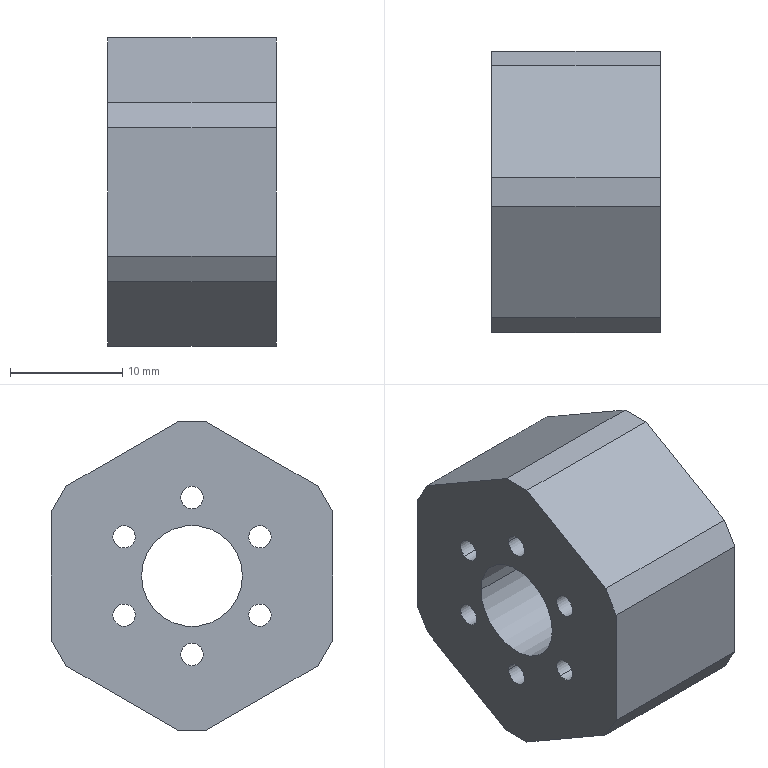Part | STEP file | ZHUANZITIEX_6_1_2_1_1 | 1 solid | 28 faces | box 15 x 25.116 x 27.5 mm | volume 6869 mm3 | plane 14 | cylinder 14 | commonest cylinder face diameters 2 x12 9 x2
STEP:
#1=CARTESIAN_POINT('',(0.,0.,0.));
#2=DIRECTION('',(0.,0.,1.));
#3=DIRECTION('',(1.,0.,0.));
#4=AXIS2_PLACEMENT_3D('',#1,#2,#3);
#5=CARTESIAN_POINT('',(0.,1.3,-13.75));
#6=VERTEX_POINT('',#5);
#7=CARTESIAN_POINT('',(0.,11.258,-8.001));
#8=VERTEX_POINT('',#7);
#9=CARTESIAN_POINT('',(0.,1.3,-13.75));
#10=DIRECTION('',(0.,0.866,0.5));
#11=VECTOR('',#10,11.498);
#12=LINE('',#9,#11);
#13=EDGE_CURVE('',#6,#8,#12,.T.);
#14=ORIENTED_EDGE('',*,*,#13,.T.);
#15=CARTESIAN_POINT('',(0.,12.558,-5.749));
#16=VERTEX_POINT('',#15);
#17=CARTESIAN_POINT('',(0.,11.258,-8.001));
#18=DIRECTION('',(0.,0.5,0.866));
#19=VECTOR('',#18,2.6);
#20=LINE('',#17,#19);
#21=EDGE_CURVE('',#8,#16,#20,.T.);
#22=ORIENTED_EDGE('',*,*,#21,.T.);
#23=CARTESIAN_POINT('',(0.,12.558,5.749));
#24=VERTEX_POINT('',#23);
#25=CARTESIAN_POINT('',(0.,12.558,-5.749));
#26=DIRECTION('',(0.,0.,1.));
#27=VECTOR('',#26,11.498);
#28=LINE('',#25,#27);
#29=EDGE_CURVE('',#16,#24,#28,.T.);
#30=ORIENTED_EDGE('',*,*,#29,.T.);
#31=CARTESIAN_POINT('',(0.,11.258,8.001));
#32=VERTEX_POINT('',#31);
#33=CARTESIAN_POINT('',(0.,12.558,5.749));
#34=DIRECTION('',(0.,-0.5,0.866));
#35=VECTOR('',#34,2.6);
#36=LINE('',#33,#35);
#37=EDGE_CURVE('',#24,#32,#36,.T.);
#38=ORIENTED_EDGE('',*,*,#37,.T.);
#39=CARTESIAN_POINT('',(0.,1.3,13.75));
#40=VERTEX_POINT('',#39);
#41=CARTESIAN_POINT('',(0.,11.258,8.001));
#42=DIRECTION('',(0.,-0.866,0.5));
#43=VECTOR('',#42,11.498);
#44=LINE('',#41,#43);
#45=EDGE_CURVE('',#32,#40,#44,.T.);
#46=ORIENTED_EDGE('',*,*,#45,.T.);
#47=CARTESIAN_POINT('',(0.,-1.3,13.75));
#48=VERTEX_POINT('',#47);
#49=CARTESIAN_POINT('',(0.,1.3,13.75));
#50=DIRECTION('',(0.,-1.,0.));
#51=VECTOR('',#50,2.6);
#52=LINE('',#49,#51);
#53=EDGE_CURVE('',#40,#48,#52,.T.);
#54=ORIENTED_EDGE('',*,*,#53,.T.);
#55=CARTESIAN_POINT('',(0.,-11.258,8.001));
#56=VERTEX_POINT('',#55);
#57=CARTESIAN_POINT('',(0.,-1.3,13.75));
#58=DIRECTION('',(0.,-0.866,-0.5));
#59=VECTOR('',#58,11.498);
#60=LINE('',#57,#59);
#61=EDGE_CURVE('',#48,#56,#60,.T.);
#62=ORIENTED_EDGE('',*,*,#61,.T.);
#63=CARTESIAN_POINT('',(0.,-12.558,5.749));
#64=VERTEX_POINT('',#63);
#65=CARTESIAN_POINT('',(0.,-11.258,8.001));
#66=DIRECTION('',(0.,-0.5,-0.866));
#67=VECTOR('',#66,2.6);
#68=LINE('',#65,#67);
#69=EDGE_CURVE('',#56,#64,#68,.T.);
#70=ORIENTED_EDGE('',*,*,#69,.T.);
#71=CARTESIAN_POINT('',(0.,-12.558,-5.749));
#72=VERTEX_POINT('',#71);
#73=CARTESIAN_POINT('',(0.,-12.558,5.749));
#74=DIRECTION('',(0.,0.,-1.));
#75=VECTOR('',#74,11.498);
#76=LINE('',#73,#75);
#77=EDGE_CURVE('',#64,#72,#76,.T.);
#78=ORIENTED_EDGE('',*,*,#77,.T.);
#79=CARTESIAN_POINT('',(0.,-11.258,-8.001));
#80=VERTEX_POINT('',#79);
#81=CARTESIAN_POINT('',(0.,-12.558,-5.749));
#82=DIRECTION('',(0.,0.5,-0.866));
#83=VECTOR('',#82,2.6);
#84=LINE('',#81,#83);
#85=EDGE_CURVE('',#72,#80,#84,.T.);
#86=ORIENTED_EDGE('',*,*,#85,.T.);
#87=CARTESIAN_POINT('',(0.,-1.3,-13.75));
#88=VERTEX_POINT('',#87);
#89=CARTESIAN_POINT('',(0.,-11.258,-8.001));
#90=DIRECTION('',(0.,0.866,-0.5));
#91=VECTOR('',#90,11.498);
#92=LINE('',#89,#91);
#93=EDGE_CURVE('',#80,#88,#92,.T.);
#94=ORIENTED_EDGE('',*,*,#93,.T.);
#95=CARTESIAN_POINT('',(0.,-1.3,-13.75));
#96=DIRECTION('',(0.,1.,0.));
#97=VECTOR('',#96,2.6);
#98=LINE('',#95,#97);
#99=EDGE_CURVE('',#88,#6,#98,.T.);
#100=ORIENTED_EDGE('',*,*,#99,.T.);
#101=EDGE_LOOP('',(#14,#22,#30,#38,#46,#54,#62,#70,#78,#86,#94,#100));
#102=FACE_OUTER_BOUND('',#101,.F.);
#103=CARTESIAN_POINT('',(0.,-4.5,0.));
#104=VERTEX_POINT('',#103);
#105=CARTESIAN_POINT('',(0.,4.5,0.));
#106=VERTEX_POINT('',#105);
#107=CARTESIAN_POINT('',(0.,0.,0.));
#108=DIRECTION('',(-1.,0.,0.));
#109=DIRECTION('',(0.,-1.,0.));
#110=AXIS2_PLACEMENT_3D('',#107,#108,#109);
#111=CIRCLE('',#110,4.5);
#112=EDGE_CURVE('',#104,#106,#111,.T.);
#113=ORIENTED_EDGE('',*,*,#112,.T.);
#114=CARTESIAN_POINT('',(0.,0.,0.));
#115=DIRECTION('',(-1.,0.,0.));
#116=DIRECTION('',(0.,1.,0.));
#117=AXIS2_PLACEMENT_3D('',#114,#115,#116);
#118=CIRCLE('',#117,4.5);
#119=EDGE_CURVE('',#106,#104,#118,.T.);
#120=ORIENTED_EDGE('',*,*,#119,.T.);
#121=EDGE_LOOP('',(#113,#120));
#122=FACE_BOUND('',#121,.F.);
#123=CARTESIAN_POINT('',(0.,1.,-7.));
#124=VERTEX_POINT('',#123);
#125=CARTESIAN_POINT('',(0.,-1.,-7.));
#126=VERTEX_POINT('',#125);
#127=CARTESIAN_POINT('',(0.,0.,-7.));
#128=DIRECTION('',(-1.,0.,0.));
#129=DIRECTION('',(0.,1.,0.));
#130=AXIS2_PLACEMENT_3D('',#127,#128,#129);
#131=CIRCLE('',#130,1.);
#132=EDGE_CURVE('',#124,#126,#131,.T.);
#133=ORIENTED_EDGE('',*,*,#132,.T.);
#134=CARTESIAN_POINT('',(0.,0.,-7.));
#135=DIRECTION('',(-1.,0.,0.));
#136=DIRECTION('',(0.,-1.,0.));
#137=AXIS2_PLACEMENT_3D('',#134,#135,#136);
#138=CIRCLE('',#137,1.);
#139=EDGE_CURVE('',#126,#124,#138,.T.);
#140=ORIENTED_EDGE('',*,*,#139,.T.);
#141=EDGE_LOOP('',(#133,#140));
#142=FACE_BOUND('',#141,.F.);
#143=CARTESIAN_POINT('',(0.,6.562,-2.634));
#144=VERTEX_POINT('',#143);
#145=CARTESIAN_POINT('',(0.,5.562,-4.366));
#146=VERTEX_POINT('',#145);
#147=CARTESIAN_POINT('',(0.,6.062,-3.5));
#148=DIRECTION('',(-1.,0.,0.));
#149=DIRECTION('',(0.,0.5,0.866));
#150=AXIS2_PLACEMENT_3D('',#147,#148,#149);
#151=CIRCLE('',#150,1.);
#152=EDGE_CURVE('',#144,#146,#151,.T.);
#153=ORIENTED_EDGE('',*,*,#152,.T.);
#154=CARTESIAN_POINT('',(0.,6.062,-3.5));
#155=DIRECTION('',(-1.,0.,0.));
#156=DIRECTION('',(0.,-0.5,-0.866));
#157=AXIS2_PLACEMENT_3D('',#154,#155,#156);
#158=CIRCLE('',#157,1.);
#159=EDGE_CURVE('',#146,#144,#158,.T.);
#160=ORIENTED_EDGE('',*,*,#159,.T.);
#161=EDGE_LOOP('',(#153,#160));
#162=FACE_BOUND('',#161,.F.);
#163=CARTESIAN_POINT('',(0.,5.562,4.366));
#164=VERTEX_POINT('',#163);
#165=CARTESIAN_POINT('',(0.,6.562,2.634));
#166=VERTEX_POINT('',#165);
#167=CARTESIAN_POINT('',(0.,6.062,3.5));
#168=DIRECTION('',(-1.,0.,0.));
#169=DIRECTION('',(0.,-0.5,0.866));
#170=AXIS2_PLACEMENT_3D('',#167,#168,#169);
#171=CIRCLE('',#170,1.);
#172=EDGE_CURVE('',#164,#166,#171,.T.);
#173=ORIENTED_EDGE('',*,*,#172,.T.);
#174=CARTESIAN_POINT('',(0.,6.062,3.5));
#175=DIRECTION('',(-1.,0.,0.));
#176=DIRECTION('',(0.,0.5,-0.866));
#177=AXIS2_PLACEMENT_3D('',#174,#175,#176);
#178=CIRCLE('',#177,1.);
#179=EDGE_CURVE('',#166,#164,#178,.T.);
#180=ORIENTED_EDGE('',*,*,#179,.T.);
#181=EDGE_LOOP('',(#173,#180));
#182=FACE_BOUND('',#181,.F.);
#183=CARTESIAN_POINT('',(0.,-1.,7.));
#184=VERTEX_POINT('',#183);
#185=CARTESIAN_POINT('',(0.,1.,7.));
#186=VERTEX_POINT('',#185);
#187=CARTESIAN_POINT('',(0.,0.,7.));
#188=DIRECTION('',(-1.,0.,0.));
#189=DIRECTION('',(0.,-1.,0.));
#190=AXIS2_PLACEMENT_3D('',#187,#188,#189);
#191=CIRCLE('',#190,1.);
#192=EDGE_CURVE('',#184,#186,#191,.T.);
#193=ORIENTED_EDGE('',*,*,#192,.T.);
#194=CARTESIAN_POINT('',(0.,0.,7.));
#195=DIRECTION('',(-1.,0.,0.));
#196=DIRECTION('',(0.,1.,0.));
#197=AXIS2_PLACEMENT_3D('',#194,#195,#196);
#198=CIRCLE('',#197,1.);
#199=EDGE_CURVE('',#186,#184,#198,.T.);
#200=ORIENTED_EDGE('',*,*,#199,.T.);
#201=EDGE_LOOP('',(#193,#200));
#202=FACE_BOUND('',#201,.F.);
#203=CARTESIAN_POINT('',(0.,-6.562,2.634));
#204=VERTEX_POINT('',#203);
#205=CARTESIAN_POINT('',(0.,-5.562,4.366));
#206=VERTEX_POINT('',#205);
#207=CARTESIAN_POINT('',(0.,-6.062,3.5));
#208=DIRECTION('',(-1.,0.,0.));
#209=DIRECTION('',(0.,-0.5,-0.866));
#210=AXIS2_PLACEMENT_3D('',#207,#208,#209);
#211=CIRCLE('',#210,1.);
#212=EDGE_CURVE('',#204,#206,#211,.T.);
#213=ORIENTED_EDGE('',*,*,#212,.T.);
#214=CARTESIAN_POINT('',(0.,-6.062,3.5));
#215=DIRECTION('',(-1.,0.,0.));
#216=DIRECTION('',(0.,0.5,0.866));
#217=AXIS2_PLACEMENT_3D('',#214,#215,#216);
#218=CIRCLE('',#217,1.);
#219=EDGE_CURVE('',#206,#204,#218,.T.);
#220=ORIENTED_EDGE('',*,*,#219,.T.);
#221=EDGE_LOOP('',(#213,#220));
#222=FACE_BOUND('',#221,.F.);
#223=CARTESIAN_POINT('',(0.,-5.562,-4.366));
#224=VERTEX_POINT('',#223);
#225=CARTESIAN_POINT('',(0.,-6.562,-2.634));
#226=VERTEX_POINT('',#225);
#227=CARTESIAN_POINT('',(0.,-6.062,-3.5));
#228=DIRECTION('',(-1.,0.,0.));
#229=DIRECTION('',(0.,0.5,-0.866));
#230=AXIS2_PLACEMENT_3D('',#227,#228,#229);
#231=CIRCLE('',#230,1.);
#232=EDGE_CURVE('',#224,#226,#231,.T.);
#233=ORIENTED_EDGE('',*,*,#232,.T.);
#234=CARTESIAN_POINT('',(0.,-6.062,-3.5));
#235=DIRECTION('',(-1.,0.,0.));
#236=DIRECTION('',(0.,-0.5,0.866));
#237=AXIS2_PLACEMENT_3D('',#234,#235,#236);
#238=CIRCLE('',#237,1.);
#239=EDGE_CURVE('',#226,#224,#238,.T.);
#240=ORIENTED_EDGE('',*,*,#239,.T.);
#241=EDGE_LOOP('',(#233,#240));
#242=FACE_BOUND('',#241,.F.);
#243=CARTESIAN_POINT('',(0.,0.,0.));
#244=DIRECTION('',(1.,0.,0.));
#245=DIRECTION('',(0.,-1.,0.));
#246=AXIS2_PLACEMENT_3D('',#243,#244,#245);
#247=PLANE('',#246);
#248=ADVANCED_FACE('',(#102,#122,#142,#162,#182,#202,#222,#242),#247,.F.);
#249=ORIENTED_EDGE('',*,*,#13,.F.);
#250=CARTESIAN_POINT('',(15.,1.3,-13.75));
#251=VERTEX_POINT('',#250);
#252=CARTESIAN_POINT('',(0.,1.3,-13.75));
#253=DIRECTION('',(1.,0.,0.));
#254=VECTOR('',#253,15.);
#255=LINE('',#252,#254);
#256=EDGE_CURVE('',#6,#251,#255,.T.);
#257=ORIENTED_EDGE('',*,*,#256,.T.);
#258=CARTESIAN_POINT('',(15.,11.258,-8.001));
#259=VERTEX_POINT('',#258);
#260=CARTESIAN_POINT('',(15.,11.258,-8.001));
#261=DIRECTION('',(0.,-0.866,-0.5));
#262=VECTOR('',#261,11.498);
#263=LINE('',#260,#262);
#264=EDGE_CURVE('',#259,#251,#263,.T.);
#265=ORIENTED_EDGE('',*,*,#264,.F.);
#266=CARTESIAN_POINT('',(0.,11.258,-8.001));
#267=DIRECTION('',(1.,0.,0.));
#268=VECTOR('',#267,15.);
#269=LINE('',#266,#268);
#270=EDGE_CURVE('',#8,#259,#269,.T.);
#271=ORIENTED_EDGE('',*,*,#270,.F.);
#272=EDGE_LOOP('',(#249,#257,#265,#271));
#273=FACE_OUTER_BOUND('',#272,.F.);
#274=CARTESIAN_POINT('',(0.,1.3,-13.75));
#275=DIRECTION('',(0.,0.5,-0.866));
#276=DIRECTION('',(0.,0.866,0.5));
#277=AXIS2_PLACEMENT_3D('',#274,#275,#276);
#278=PLANE('',#277);
#279=ADVANCED_FACE('',(#273),#278,.T.);
#280=ORIENTED_EDGE('',*,*,#99,.F.);
#281=CARTESIAN_POINT('',(15.,-1.3,-13.75));
#282=VERTEX_POINT('',#281);
#283=CARTESIAN_POINT('',(0.,-1.3,-13.75));
#284=DIRECTION('',(1.,0.,0.));
#285=VECTOR('',#284,15.);
#286=LINE('',#283,#285);
#287=EDGE_CURVE('',#88,#282,#286,.T.);
#288=ORIENTED_EDGE('',*,*,#287,.T.);
#289=CARTESIAN_POINT('',(15.,-1.3,-13.75));
#290=DIRECTION('',(0.,1.,0.));
#291=VECTOR('',#290,2.6);
#292=LINE('',#289,#291);
#293=EDGE_CURVE('',#282,#251,#292,.T.);
#294=ORIENTED_EDGE('',*,*,#293,.T.);
#295=ORIENTED_EDGE('',*,*,#256,.F.);
#296=EDGE_LOOP('',(#280,#288,#294,#295));
#297=FACE_OUTER_BOUND('',#296,.F.);
#298=CARTESIAN_POINT('',(0.,-1.3,-13.75));
#299=DIRECTION('',(0.,0.,-1.));
#300=DIRECTION('',(0.,1.,0.));
#301=AXIS2_PLACEMENT_3D('',#298,#299,#300);
#302=PLANE('',#301);
#303=ADVANCED_FACE('',(#297),#302,.T.);
#304=ORIENTED_EDGE('',*,*,#93,.F.);
#305=CARTESIAN_POINT('',(15.,-11.258,-8.001));
#306=VERTEX_POINT('',#305);
#307=CARTESIAN_POINT('',(0.,-11.258,-8.001));
#308=DIRECTION('',(1.,0.,0.));
#309=VECTOR('',#308,15.);
#310=LINE('',#307,#309);
#311=EDGE_CURVE('',#80,#306,#310,.T.);
#312=ORIENTED_EDGE('',*,*,#311,.T.);
#313=CARTESIAN_POINT('',(15.,-1.3,-13.75));
#314=DIRECTION('',(0.,-0.866,0.5));
#315=VECTOR('',#314,11.498);
#316=LINE('',#313,#315);
#317=EDGE_CURVE('',#282,#306,#316,.T.);
#318=ORIENTED_EDGE('',*,*,#317,.F.);
#319=ORIENTED_EDGE('',*,*,#287,.F.);
#320=EDGE_LOOP('',(#304,#312,#318,#319));
#321=FACE_OUTER_BOUND('',#320,.F.);
#322=CARTESIAN_POINT('',(0.,-11.258,-8.001));
#323=DIRECTION('',(0.,-0.5,-0.866));
#324=DIRECTION('',(0.,0.866,-0.5));
#325=AXIS2_PLACEMENT_3D('',#322,#323,#324);
#326=PLANE('',#325);
#327=ADVANCED_FACE('',(#321),#326,.T.);
#328=ORIENTED_EDGE('',*,*,#85,.F.);
#329=CARTESIAN_POINT('',(15.,-12.558,-5.749));
#330=VERTEX_POINT('',#329);
#331=CARTESIAN_POINT('',(0.,-12.558,-5.749));
#332=DIRECTION('',(1.,0.,0.));
#333=VECTOR('',#332,15.);
#334=LINE('',#331,#333);
#335=EDGE_CURVE('',#72,#330,#334,.T.);
#336=ORIENTED_EDGE('',*,*,#335,.T.);
#337=CARTESIAN_POINT('',(15.,-11.258,-8.001));
#338=DIRECTION('',(0.,-0.5,0.866));
#339=VECTOR('',#338,2.6);
#340=LINE('',#337,#339);
#341=EDGE_CURVE('',#306,#330,#340,.T.);
#342=ORIENTED_EDGE('',*,*,#341,.F.);
#343=ORIENTED_EDGE('',*,*,#311,.F.);
#344=EDGE_LOOP('',(#328,#336,#342,#343));
#345=FACE_OUTER_BOUND('',#344,.F.);
#346=CARTESIAN_POINT('',(0.,-12.558,-5.749));
#347=DIRECTION('',(0.,-0.866,-0.5));
#348=DIRECTION('',(0.,0.5,-0.866));
#349=AXIS2_PLACEMENT_3D('',#346,#347,#348);
#350=PLANE('',#349);
#351=ADVANCED_FACE('',(#345),#350,.T.);
#352=ORIENTED_EDGE('',*,*,#77,.F.);
#353=CARTESIAN_POINT('',(15.,-12.558,5.749));
#354=VERTEX_POINT('',#353);
#355=CARTESIAN_POINT('',(0.,-12.558,5.749));
#356=DIRECTION('',(1.,0.,0.));
#357=VECTOR('',#356,15.);
#358=LINE('',#355,#357);
#359=EDGE_CURVE('',#64,#354,#358,.T.);
#360=ORIENTED_EDGE('',*,*,#359,.T.);
#361=CARTESIAN_POINT('',(15.,-12.558,5.749));
#362=DIRECTION('',(0.,0.,-1.));
#363=VECTOR('',#362,11.498);
#364=LINE('',#361,#363);
#365=EDGE_CURVE('',#354,#330,#364,.T.);
#366=ORIENTED_EDGE('',*,*,#365,.T.);
#367=ORIENTED_EDGE('',*,*,#335,.F.);
#368=EDGE_LOOP('',(#352,#360,#366,#367));
#369=FACE_OUTER_BOUND('',#368,.F.);
#370=CARTESIAN_POINT('',(0.,-12.558,5.749));
#371=DIRECTION('',(0.,-1.,0.));
#372=DIRECTION('',(0.,0.,-1.));
#373=AXIS2_PLACEMENT_3D('',#370,#371,#372);
#374=PLANE('',#373);
#375=ADVANCED_FACE('',(#369),#374,.T.);
#376=ORIENTED_EDGE('',*,*,#69,.F.);
#377=CARTESIAN_POINT('',(15.,-11.258,8.001));
#378=VERTEX_POINT('',#377);
#379=CARTESIAN_POINT('',(0.,-11.258,8.001));
#380=DIRECTION('',(1.,0.,0.));
#381=VECTOR('',#380,15.);
#382=LINE('',#379,#381);
#383=EDGE_CURVE('',#56,#378,#382,.T.);
#384=ORIENTED_EDGE('',*,*,#383,.T.);
#385=CARTESIAN_POINT('',(15.,-12.558,5.749));
#386=DIRECTION('',(0.,0.5,0.866));
#387=VECTOR('',#386,2.6);
#388=LINE('',#385,#387);
#389=EDGE_CURVE('',#354,#378,#388,.T.);
#390=ORIENTED_EDGE('',*,*,#389,.F.);
#391=ORIENTED_EDGE('',*,*,#359,.F.);
#392=EDGE_LOOP('',(#376,#384,#390,#391));
#393=FACE_OUTER_BOUND('',#392,.F.);
#394=CARTESIAN_POINT('',(0.,-11.258,8.001));
#395=DIRECTION('',(0.,-0.866,0.5));
#396=DIRECTION('',(0.,-0.5,-0.866));
#397=AXIS2_PLACEMENT_3D('',#394,#395,#396);
#398=PLANE('',#397);
#399=ADVANCED_FACE('',(#393),#398,.T.);
#400=ORIENTED_EDGE('',*,*,#61,.F.);
#401=CARTESIAN_POINT('',(15.,-1.3,13.75));
#402=VERTEX_POINT('',#401);
#403=CARTESIAN_POINT('',(0.,-1.3,13.75));
#404=DIRECTION('',(1.,0.,0.));
#405=VECTOR('',#404,15.);
#406=LINE('',#403,#405);
#407=EDGE_CURVE('',#48,#402,#406,.T.);
#408=ORIENTED_EDGE('',*,*,#407,.T.);
#409=CARTESIAN_POINT('',(15.,-11.258,8.001));
#410=DIRECTION('',(0.,0.866,0.5));
#411=VECTOR('',#410,11.498);
#412=LINE('',#409,#411);
#413=EDGE_CURVE('',#378,#402,#412,.T.);
#414=ORIENTED_EDGE('',*,*,#413,.F.);
#415=ORIENTED_EDGE('',*,*,#383,.F.);
#416=EDGE_LOOP('',(#400,#408,#414,#415));
#417=FACE_OUTER_BOUND('',#416,.F.);
#418=CARTESIAN_POINT('',(0.,-1.3,13.75));
#419=DIRECTION('',(0.,-0.5,0.866));
#420=DIRECTION('',(0.,-0.866,-0.5));
#421=AXIS2_PLACEMENT_3D('',#418,#419,#420);
#422=PLANE('',#421);
#423=ADVANCED_FACE('',(#417),#422,.T.);
#424=ORIENTED_EDGE('',*,*,#53,.F.);
#425=CARTESIAN_POINT('',(15.,1.3,13.75));
#426=VERTEX_POINT('',#425);
#427=CARTESIAN_POINT('',(0.,1.3,13.75));
#428=DIRECTION('',(1.,0.,0.));
#429=VECTOR('',#428,15.);
#430=LINE('',#427,#429);
#431=EDGE_CURVE('',#40,#426,#430,.T.);
#432=ORIENTED_EDGE('',*,*,#431,.T.);
#433=CARTESIAN_POINT('',(15.,1.3,13.75));
#434=DIRECTION('',(0.,-1.,0.));
#435=VECTOR('',#434,2.6);
#436=LINE('',#433,#435);
#437=EDGE_CURVE('',#426,#402,#436,.T.);
#438=ORIENTED_EDGE('',*,*,#437,.T.);
#439=ORIENTED_EDGE('',*,*,#407,.F.);
#440=EDGE_LOOP('',(#424,#432,#438,#439));
#441=FACE_OUTER_BOUND('',#440,.F.);
#442=CARTESIAN_POINT('',(0.,1.3,13.75));
#443=DIRECTION('',(0.,0.,1.));
#444=DIRECTION('',(0.,-1.,0.));
#445=AXIS2_PLACEMENT_3D('',#442,#443,#444);
#446=PLANE('',#445);
#447=ADVANCED_FACE('',(#441),#446,.T.);
#448=ORIENTED_EDGE('',*,*,#45,.F.);
#449=CARTESIAN_POINT('',(15.,11.258,8.001));
#450=VERTEX_POINT('',#449);
#451=CARTESIAN_POINT('',(0.,11.258,8.001));
#452=DIRECTION('',(1.,0.,0.));
#453=VECTOR('',#452,15.);
#454=LINE('',#451,#453);
#455=EDGE_CURVE('',#32,#450,#454,.T.);
#456=ORIENTED_EDGE('',*,*,#455,.T.);
#457=CARTESIAN_POINT('',(15.,1.3,13.75));
#458=DIRECTION('',(0.,0.866,-0.5));
#459=VECTOR('',#458,11.498);
#460=LINE('',#457,#459);
#461=EDGE_CURVE('',#426,#450,#460,.T.);
#462=ORIENTED_EDGE('',*,*,#461,.F.);
#463=ORIENTED_EDGE('',*,*,#431,.F.);
#464=EDGE_LOOP('',(#448,#456,#462,#463));
#465=FACE_OUTER_BOUND('',#464,.F.);
#466=CARTESIAN_POINT('',(0.,11.258,8.001));
#467=DIRECTION('',(0.,0.5,0.866));
#468=DIRECTION('',(0.,-0.866,0.5));
#469=AXIS2_PLACEMENT_3D('',#466,#467,#468);
#470=PLANE('',#469);
#471=ADVANCED_FACE('',(#465),#470,.T.);
#472=ORIENTED_EDGE('',*,*,#37,.F.);
#473=CARTESIAN_POINT('',(15.,12.558,5.749));
#474=VERTEX_POINT('',#473);
#475=CARTESIAN_POINT('',(0.,12.558,5.749));
#476=DIRECTION('',(1.,0.,0.));
#477=VECTOR('',#476,15.);
#478=LINE('',#475,#477);
#479=EDGE_CURVE('',#24,#474,#478,.T.);
#480=ORIENTED_EDGE('',*,*,#479,.T.);
#481=CARTESIAN_POINT('',(15.,11.258,8.001));
#482=DIRECTION('',(0.,0.5,-0.866));
#483=VECTOR('',#482,2.6);
#484=LINE('',#481,#483);
#485=EDGE_CURVE('',#450,#474,#484,.T.);
#486=ORIENTED_EDGE('',*,*,#485,.F.);
#487=ORIENTED_EDGE('',*,*,#455,.F.);
#488=EDGE_LOOP('',(#472,#480,#486,#487));
#489=FACE_OUTER_BOUND('',#488,.F.);
#490=CARTESIAN_POINT('',(0.,12.558,5.749));
#491=DIRECTION('',(0.,0.866,0.5));
#492=DIRECTION('',(0.,-0.5,0.866));
#493=AXIS2_PLACEMENT_3D('',#490,#491,#492);
#494=PLANE('',#493);
#495=ADVANCED_FACE('',(#489),#494,.T.);
#496=ORIENTED_EDGE('',*,*,#29,.F.);
#497=CARTESIAN_POINT('',(15.,12.558,-5.749));
#498=VERTEX_POINT('',#497);
#499=CARTESIAN_POINT('',(0.,12.558,-5.749));
#500=DIRECTION('',(1.,0.,0.));
#501=VECTOR('',#500,15.);
#502=LINE('',#499,#501);
#503=EDGE_CURVE('',#16,#498,#502,.T.);
#504=ORIENTED_EDGE('',*,*,#503,.T.);
#505=CARTESIAN_POINT('',(15.,12.558,-5.749));
#506=DIRECTION('',(0.,0.,1.));
#507=VECTOR('',#506,11.498);
#508=LINE('',#505,#507);
#509=EDGE_CURVE('',#498,#474,#508,.T.);
#510=ORIENTED_EDGE('',*,*,#509,.T.);
#511=ORIENTED_EDGE('',*,*,#479,.F.);
#512=EDGE_LOOP('',(#496,#504,#510,#511));
#513=FACE_OUTER_BOUND('',#512,.F.);
#514=CARTESIAN_POINT('',(0.,12.558,-5.749));
#515=DIRECTION('',(0.,1.,0.));
#516=DIRECTION('',(0.,0.,1.));
#517=AXIS2_PLACEMENT_3D('',#514,#515,#516);
#518=PLANE('',#517);
#519=ADVANCED_FACE('',(#513),#518,.T.);
#520=ORIENTED_EDGE('',*,*,#21,.F.);
#521=ORIENTED_EDGE('',*,*,#270,.T.);
#522=CARTESIAN_POINT('',(15.,12.558,-5.749));
#523=DIRECTION('',(0.,-0.5,-0.866));
#524=VECTOR('',#523,2.6);
#525=LINE('',#522,#524);
#526=EDGE_CURVE('',#498,#259,#525,.T.);
#527=ORIENTED_EDGE('',*,*,#526,.F.);
#528=ORIENTED_EDGE('',*,*,#503,.F.);
#529=EDGE_LOOP('',(#520,#521,#527,#528));
#530=FACE_OUTER_BOUND('',#529,.F.);
#531=CARTESIAN_POINT('',(0.,11.258,-8.001));
#532=DIRECTION('',(0.,0.866,-0.5));
#533=DIRECTION('',(0.,0.5,0.866));
#534=AXIS2_PLACEMENT_3D('',#531,#532,#533);
#535=PLANE('',#534);
#536=ADVANCED_FACE('',(#530),#535,.T.);
#537=ORIENTED_EDGE('',*,*,#264,.T.);
#538=ORIENTED_EDGE('',*,*,#293,.F.);
#539=ORIENTED_EDGE('',*,*,#317,.T.);
#540=ORIENTED_EDGE('',*,*,#341,.T.);
#541=ORIENTED_EDGE('',*,*,#365,.F.);
#542=ORIENTED_EDGE('',*,*,#389,.T.);
#543=ORIENTED_EDGE('',*,*,#413,.T.);
#544=ORIENTED_EDGE('',*,*,#437,.F.);
#545=ORIENTED_EDGE('',*,*,#461,.T.);
#546=ORIENTED_EDGE('',*,*,#485,.T.);
#547=ORIENTED_EDGE('',*,*,#509,.F.);
#548=ORIENTED_EDGE('',*,*,#526,.T.);
#549=EDGE_LOOP('',(#537,#538,#539,#540,#541,#542,#543,#544,#545,#546,#547,#548));
#550=FACE_OUTER_BOUND('',#549,.F.);
#551=CARTESIAN_POINT('',(15.,4.5,0.));
#552=VERTEX_POINT('',#551);
#553=CARTESIAN_POINT('',(15.,-4.5,0.));
#554=VERTEX_POINT('',#553);
#555=CARTESIAN_POINT('',(15.,0.,0.));
#556=DIRECTION('',(1.,0.,0.));
#557=DIRECTION('',(0.,1.,0.));
#558=AXIS2_PLACEMENT_3D('',#555,#556,#557);
#559=CIRCLE('',#558,4.5);
#560=EDGE_CURVE('',#552,#554,#559,.T.);
#561=ORIENTED_EDGE('',*,*,#560,.T.);
#562=CARTESIAN_POINT('',(15.,0.,0.));
#563=DIRECTION('',(1.,0.,0.));
#564=DIRECTION('',(0.,-1.,0.));
#565=AXIS2_PLACEMENT_3D('',#562,#563,#564);
#566=CIRCLE('',#565,4.5);
#567=EDGE_CURVE('',#554,#552,#566,.T.);
#568=ORIENTED_EDGE('',*,*,#567,.T.);
#569=EDGE_LOOP('',(#561,#568));
#570=FACE_BOUND('',#569,.F.);
#571=CARTESIAN_POINT('',(15.,-1.,-7.));
#572=VERTEX_POINT('',#571);
#573=CARTESIAN_POINT('',(15.,1.,-7.));
#574=VERTEX_POINT('',#573);
#575=CARTESIAN_POINT('',(15.,0.,-7.));
#576=DIRECTION('',(1.,0.,0.));
#577=DIRECTION('',(0.,-1.,0.));
#578=AXIS2_PLACEMENT_3D('',#575,#576,#577);
#579=CIRCLE('',#578,1.);
#580=EDGE_CURVE('',#572,#574,#579,.T.);
#581=ORIENTED_EDGE('',*,*,#580,.T.);
#582=CARTESIAN_POINT('',(15.,0.,-7.));
#583=DIRECTION('',(1.,0.,0.));
#584=DIRECTION('',(0.,1.,0.));
#585=AXIS2_PLACEMENT_3D('',#582,#583,#584);
#586=CIRCLE('',#585,1.);
#587=EDGE_CURVE('',#574,#572,#586,.T.);
#588=ORIENTED_EDGE('',*,*,#587,.T.);
#589=EDGE_LOOP('',(#581,#588));
#590=FACE_BOUND('',#589,.F.);
#591=CARTESIAN_POINT('',(15.,5.562,-4.366));
#592=VERTEX_POINT('',#591);
#593=CARTESIAN_POINT('',(15.,6.562,-2.634));
#594=VERTEX_POINT('',#593);
#595=CARTESIAN_POINT('',(15.,6.062,-3.5));
#596=DIRECTION('',(1.,0.,0.));
#597=DIRECTION('',(0.,-0.5,-0.866));
#598=AXIS2_PLACEMENT_3D('',#595,#596,#597);
#599=CIRCLE('',#598,1.);
#600=EDGE_CURVE('',#592,#594,#599,.T.);
#601=ORIENTED_EDGE('',*,*,#600,.T.);
#602=CARTESIAN_POINT('',(15.,6.062,-3.5));
#603=DIRECTION('',(1.,0.,0.));
#604=DIRECTION('',(0.,0.5,0.866));
#605=AXIS2_PLACEMENT_3D('',#602,#603,#604);
#606=CIRCLE('',#605,1.);
#607=EDGE_CURVE('',#594,#592,#606,.T.);
#608=ORIENTED_EDGE('',*,*,#607,.T.);
#609=EDGE_LOOP('',(#601,#608));
#610=FACE_BOUND('',#609,.F.);
#611=CARTESIAN_POINT('',(15.,6.562,2.634));
#612=VERTEX_POINT('',#611);
#613=CARTESIAN_POINT('',(15.,5.562,4.366));
#614=VERTEX_POINT('',#613);
#615=CARTESIAN_POINT('',(15.,6.062,3.5));
#616=DIRECTION('',(1.,0.,0.));
#617=DIRECTION('',(0.,0.5,-0.866));
#618=AXIS2_PLACEMENT_3D('',#615,#616,#617);
#619=CIRCLE('',#618,1.);
#620=EDGE_CURVE('',#612,#614,#619,.T.);
#621=ORIENTED_EDGE('',*,*,#620,.T.);
#622=CARTESIAN_POINT('',(15.,6.062,3.5));
#623=DIRECTION('',(1.,0.,0.));
#624=DIRECTION('',(0.,-0.5,0.866));
#625=AXIS2_PLACEMENT_3D('',#622,#623,#624);
#626=CIRCLE('',#625,1.);
#627=EDGE_CURVE('',#614,#612,#626,.T.);
#628=ORIENTED_EDGE('',*,*,#627,.T.);
#629=EDGE_LOOP('',(#621,#628));
#630=FACE_BOUND('',#629,.F.);
#631=CARTESIAN_POINT('',(15.,1.,7.));
#632=VERTEX_POINT('',#631);
#633=CARTESIAN_POINT('',(15.,-1.,7.));
#634=VERTEX_POINT('',#633);
#635=CARTESIAN_POINT('',(15.,0.,7.));
#636=DIRECTION('',(1.,0.,0.));
#637=DIRECTION('',(0.,1.,0.));
#638=AXIS2_PLACEMENT_3D('',#635,#636,#637);
#639=CIRCLE('',#638,1.);
#640=EDGE_CURVE('',#632,#634,#639,.T.);
#641=ORIENTED_EDGE('',*,*,#640,.T.);
#642=CARTESIAN_POINT('',(15.,0.,7.));
#643=DIRECTION('',(1.,0.,0.));
#644=DIRECTION('',(0.,-1.,0.));
#645=AXIS2_PLACEMENT_3D('',#642,#643,#644);
#646=CIRCLE('',#645,1.);
#647=EDGE_CURVE('',#634,#632,#646,.T.);
#648=ORIENTED_EDGE('',*,*,#647,.T.);
#649=EDGE_LOOP('',(#641,#648));
#650=FACE_BOUND('',#649,.F.);
#651=CARTESIAN_POINT('',(15.,-5.562,4.366));
#652=VERTEX_POINT('',#651);
#653=CARTESIAN_POINT('',(15.,-6.562,2.634));
#654=VERTEX_POINT('',#653);
#655=CARTESIAN_POINT('',(15.,-6.062,3.5));
#656=DIRECTION('',(1.,0.,0.));
#657=DIRECTION('',(0.,0.5,0.866));
#658=AXIS2_PLACEMENT_3D('',#655,#656,#657);
#659=CIRCLE('',#658,1.);
#660=EDGE_CURVE('',#652,#654,#659,.T.);
#661=ORIENTED_EDGE('',*,*,#660,.T.);
#662=CARTESIAN_POINT('',(15.,-6.062,3.5));
#663=DIRECTION('',(1.,0.,0.));
#664=DIRECTION('',(0.,-0.5,-0.866));
#665=AXIS2_PLACEMENT_3D('',#662,#663,#664);
#666=CIRCLE('',#665,1.);
#667=EDGE_CURVE('',#654,#652,#666,.T.);
#668=ORIENTED_EDGE('',*,*,#667,.T.);
#669=EDGE_LOOP('',(#661,#668));
#670=FACE_BOUND('',#669,.F.);
#671=CARTESIAN_POINT('',(15.,-6.562,-2.634));
#672=VERTEX_POINT('',#671);
#673=CARTESIAN_POINT('',(15.,-5.562,-4.366));
#674=VERTEX_POINT('',#673);
#675=CARTESIAN_POINT('',(15.,-6.062,-3.5));
#676=DIRECTION('',(1.,0.,0.));
#677=DIRECTION('',(0.,-0.5,0.866));
#678=AXIS2_PLACEMENT_3D('',#675,#676,#677);
#679=CIRCLE('',#678,1.);
#680=EDGE_CURVE('',#672,#674,#679,.T.);
#681=ORIENTED_EDGE('',*,*,#680,.T.);
#682=CARTESIAN_POINT('',(15.,-6.062,-3.5));
#683=DIRECTION('',(1.,0.,0.));
#684=DIRECTION('',(0.,0.5,-0.866));
#685=AXIS2_PLACEMENT_3D('',#682,#683,#684);
#686=CIRCLE('',#685,1.);
#687=EDGE_CURVE('',#674,#672,#686,.T.);
#688=ORIENTED_EDGE('',*,*,#687,.T.);
#689=EDGE_LOOP('',(#681,#688));
#690=FACE_BOUND('',#689,.F.);
#691=CARTESIAN_POINT('',(15.,0.,0.));
#692=DIRECTION('',(1.,0.,0.));
#693=DIRECTION('',(0.,-1.,0.));
#694=AXIS2_PLACEMENT_3D('',#691,#692,#693);
#695=PLANE('',#694);
#696=ADVANCED_FACE('',(#550,#570,#590,#610,#630,#650,#670,#690),#695,.T.);
#697=ORIENTED_EDGE('',*,*,#112,.F.);
#698=CARTESIAN_POINT('',(0.,-4.5,0.));
#699=DIRECTION('',(1.,0.,0.));
#700=VECTOR('',#699,15.);
#701=LINE('',#698,#700);
#702=EDGE_CURVE('',#104,#554,#701,.T.);
#703=ORIENTED_EDGE('',*,*,#702,.T.);
#704=ORIENTED_EDGE('',*,*,#560,.F.);
#705=CARTESIAN_POINT('',(0.,4.5,0.));
#706=DIRECTION('',(1.,0.,0.));
#707=VECTOR('',#706,15.);
#708=LINE('',#705,#707);
#709=EDGE_CURVE('',#106,#552,#708,.T.);
#710=ORIENTED_EDGE('',*,*,#709,.F.);
#711=EDGE_LOOP('',(#697,#703,#704,#710));
#712=FACE_OUTER_BOUND('',#711,.F.);
#713=CARTESIAN_POINT('',(0.,0.,0.));
#714=DIRECTION('',(1.,0.,0.));
#715=DIRECTION('',(0.,-1.,0.));
#716=AXIS2_PLACEMENT_3D('',#713,#714,#715);
#717=CYLINDRICAL_SURFACE('',#716,4.5);
#718=ADVANCED_FACE('',(#712),#717,.F.);
#719=ORIENTED_EDGE('',*,*,#119,.F.);
#720=ORIENTED_EDGE('',*,*,#709,.T.);
#721=ORIENTED_EDGE('',*,*,#567,.F.);
#722=ORIENTED_EDGE('',*,*,#702,.F.);
#723=EDGE_LOOP('',(#719,#720,#721,#722));
#724=FACE_OUTER_BOUND('',#723,.F.);
#725=CARTESIAN_POINT('',(0.,0.,0.));
#726=DIRECTION('',(1.,0.,0.));
#727=DIRECTION('',(0.,-1.,0.));
#728=AXIS2_PLACEMENT_3D('',#725,#726,#727);
#729=CYLINDRICAL_SURFACE('',#728,4.5);
#730=ADVANCED_FACE('',(#724),#729,.F.);
#731=ORIENTED_EDGE('',*,*,#132,.F.);
#732=CARTESIAN_POINT('',(15.,1.,-7.));
#733=DIRECTION('',(-1.,0.,0.));
#734=VECTOR('',#733,15.);
#735=LINE('',#732,#734);
#736=EDGE_CURVE('',#574,#124,#735,.T.);
#737=ORIENTED_EDGE('',*,*,#736,.F.);
#738=ORIENTED_EDGE('',*,*,#580,.F.);
#739=CARTESIAN_POINT('',(15.,-1.,-7.));
#740=DIRECTION('',(-1.,0.,0.));
#741=VECTOR('',#740,15.);
#742=LINE('',#739,#741);
#743=EDGE_CURVE('',#572,#126,#742,.T.);
#744=ORIENTED_EDGE('',*,*,#743,.T.);
#745=EDGE_LOOP('',(#731,#737,#738,#744));
#746=FACE_OUTER_BOUND('',#745,.F.);
#747=CARTESIAN_POINT('',(15.,0.,-7.));
#748=DIRECTION('',(1.,0.,0.));
#749=DIRECTION('',(0.,-1.,0.));
#750=AXIS2_PLACEMENT_3D('',#747,#748,#749);
#751=CYLINDRICAL_SURFACE('',#750,1.);
#752=ADVANCED_FACE('',(#746),#751,.F.);
#753=ORIENTED_EDGE('',*,*,#139,.F.);
#754=ORIENTED_EDGE('',*,*,#743,.F.);
#755=ORIENTED_EDGE('',*,*,#587,.F.);
#756=ORIENTED_EDGE('',*,*,#736,.T.);
#757=EDGE_LOOP('',(#753,#754,#755,#756));
#758=FACE_OUTER_BOUND('',#757,.F.);
#759=CARTESIAN_POINT('',(15.,0.,-7.));
#760=DIRECTION('',(1.,0.,0.));
#761=DIRECTION('',(0.,-1.,0.));
#762=AXIS2_PLACEMENT_3D('',#759,#760,#761);
#763=CYLINDRICAL_SURFACE('',#762,1.);
#764=ADVANCED_FACE('',(#758),#763,.F.);
#765=ORIENTED_EDGE('',*,*,#152,.F.);
#766=CARTESIAN_POINT('',(15.,6.562,-2.634));
#767=DIRECTION('',(-1.,0.,0.));
#768=VECTOR('',#767,15.);
#769=LINE('',#766,#768);
#770=EDGE_CURVE('',#594,#144,#769,.T.);
#771=ORIENTED_EDGE('',*,*,#770,.F.);
#772=ORIENTED_EDGE('',*,*,#600,.F.);
#773=CARTESIAN_POINT('',(15.,5.562,-4.366));
#774=DIRECTION('',(-1.,0.,0.));
#775=VECTOR('',#774,15.);
#776=LINE('',#773,#775);
#777=EDGE_CURVE('',#592,#146,#776,.T.);
#778=ORIENTED_EDGE('',*,*,#777,.T.);
#779=EDGE_LOOP('',(#765,#771,#772,#778));
#780=FACE_OUTER_BOUND('',#779,.F.);
#781=CARTESIAN_POINT('',(15.,6.062,-3.5));
#782=DIRECTION('',(1.,0.,0.));
#783=DIRECTION('',(0.,-0.5,-0.866));
#784=AXIS2_PLACEMENT_3D('',#781,#782,#783);
#785=CYLINDRICAL_SURFACE('',#784,1.);
#786=ADVANCED_FACE('',(#780),#785,.F.);
#787=ORIENTED_EDGE('',*,*,#159,.F.);
#788=ORIENTED_EDGE('',*,*,#777,.F.);
#789=ORIENTED_EDGE('',*,*,#607,.F.);
#790=ORIENTED_EDGE('',*,*,#770,.T.);
#791=EDGE_LOOP('',(#787,#788,#789,#790));
#792=FACE_OUTER_BOUND('',#791,.F.);
#793=CARTESIAN_POINT('',(15.,6.062,-3.5));
#794=DIRECTION('',(1.,0.,0.));
#795=DIRECTION('',(0.,-0.5,-0.866));
#796=AXIS2_PLACEMENT_3D('',#793,#794,#795);
#797=CYLINDRICAL_SURFACE('',#796,1.);
#798=ADVANCED_FACE('',(#792),#797,.F.);
#799=ORIENTED_EDGE('',*,*,#172,.F.);
#800=CARTESIAN_POINT('',(15.,5.562,4.366));
#801=DIRECTION('',(-1.,0.,0.));
#802=VECTOR('',#801,15.);
#803=LINE('',#800,#802);
#804=EDGE_CURVE('',#614,#164,#803,.T.);
#805=ORIENTED_EDGE('',*,*,#804,.F.);
#806=ORIENTED_EDGE('',*,*,#620,.F.);
#807=CARTESIAN_POINT('',(15.,6.562,2.634));
#808=DIRECTION('',(-1.,0.,0.));
#809=VECTOR('',#808,15.);
#810=LINE('',#807,#809);
#811=EDGE_CURVE('',#612,#166,#810,.T.);
#812=ORIENTED_EDGE('',*,*,#811,.T.);
#813=EDGE_LOOP('',(#799,#805,#806,#812));
#814=FACE_OUTER_BOUND('',#813,.F.);
#815=CARTESIAN_POINT('',(15.,6.062,3.5));
#816=DIRECTION('',(1.,0.,0.));
#817=DIRECTION('',(0.,0.5,-0.866));
#818=AXIS2_PLACEMENT_3D('',#815,#816,#817);
#819=CYLINDRICAL_SURFACE('',#818,1.);
#820=ADVANCED_FACE('',(#814),#819,.F.);
#821=ORIENTED_EDGE('',*,*,#179,.F.);
#822=ORIENTED_EDGE('',*,*,#811,.F.);
#823=ORIENTED_EDGE('',*,*,#627,.F.);
#824=ORIENTED_EDGE('',*,*,#804,.T.);
#825=EDGE_LOOP('',(#821,#822,#823,#824));
#826=FACE_OUTER_BOUND('',#825,.F.);
#827=CARTESIAN_POINT('',(15.,6.062,3.5));
#828=DIRECTION('',(1.,0.,0.));
#829=DIRECTION('',(0.,0.5,-0.866));
#830=AXIS2_PLACEMENT_3D('',#827,#828,#829);
#831=CYLINDRICAL_SURFACE('',#830,1.);
#832=ADVANCED_FACE('',(#826),#831,.F.);
#833=ORIENTED_EDGE('',*,*,#192,.F.);
#834=CARTESIAN_POINT('',(15.,-1.,7.));
#835=DIRECTION('',(-1.,0.,0.));
#836=VECTOR('',#835,15.);
#837=LINE('',#834,#836);
#838=EDGE_CURVE('',#634,#184,#837,.T.);
#839=ORIENTED_EDGE('',*,*,#838,.F.);
#840=ORIENTED_EDGE('',*,*,#640,.F.);
#841=CARTESIAN_POINT('',(15.,1.,7.));
#842=DIRECTION('',(-1.,0.,0.));
#843=VECTOR('',#842,15.);
#844=LINE('',#841,#843);
#845=EDGE_CURVE('',#632,#186,#844,.T.);
#846=ORIENTED_EDGE('',*,*,#845,.T.);
#847=EDGE_LOOP('',(#833,#839,#840,#846));
#848=FACE_OUTER_BOUND('',#847,.F.);
#849=CARTESIAN_POINT('',(15.,0.,7.));
#850=DIRECTION('',(1.,0.,0.));
#851=DIRECTION('',(0.,1.,0.));
#852=AXIS2_PLACEMENT_3D('',#849,#850,#851);
#853=CYLINDRICAL_SURFACE('',#852,1.);
#854=ADVANCED_FACE('',(#848),#853,.F.);
#855=ORIENTED_EDGE('',*,*,#199,.F.);
#856=ORIENTED_EDGE('',*,*,#845,.F.);
#857=ORIENTED_EDGE('',*,*,#647,.F.);
#858=ORIENTED_EDGE('',*,*,#838,.T.);
#859=EDGE_LOOP('',(#855,#856,#857,#858));
#860=FACE_OUTER_BOUND('',#859,.F.);
#861=CARTESIAN_POINT('',(15.,0.,7.));
#862=DIRECTION('',(1.,0.,0.));
#863=DIRECTION('',(0.,1.,0.));
#864=AXIS2_PLACEMENT_3D('',#861,#862,#863);
#865=CYLINDRICAL_SURFACE('',#864,1.);
#866=ADVANCED_FACE('',(#860),#865,.F.);
#867=ORIENTED_EDGE('',*,*,#212,.F.);
#868=CARTESIAN_POINT('',(15.,-6.562,2.634));
#869=DIRECTION('',(-1.,0.,0.));
#870=VECTOR('',#869,15.);
#871=LINE('',#868,#870);
#872=EDGE_CURVE('',#654,#204,#871,.T.);
#873=ORIENTED_EDGE('',*,*,#872,.F.);
#874=ORIENTED_EDGE('',*,*,#660,.F.);
#875=CARTESIAN_POINT('',(15.,-5.562,4.366));
#876=DIRECTION('',(-1.,0.,0.));
#877=VECTOR('',#876,15.);
#878=LINE('',#875,#877);
#879=EDGE_CURVE('',#652,#206,#878,.T.);
#880=ORIENTED_EDGE('',*,*,#879,.T.);
#881=EDGE_LOOP('',(#867,#873,#874,#880));
#882=FACE_OUTER_BOUND('',#881,.F.);
#883=CARTESIAN_POINT('',(15.,-6.062,3.5));
#884=DIRECTION('',(1.,0.,0.));
#885=DIRECTION('',(0.,0.5,0.866));
#886=AXIS2_PLACEMENT_3D('',#883,#884,#885);
#887=CYLINDRICAL_SURFACE('',#886,1.);
#888=ADVANCED_FACE('',(#882),#887,.F.);
#889=ORIENTED_EDGE('',*,*,#219,.F.);
#890=ORIENTED_EDGE('',*,*,#879,.F.);
#891=ORIENTED_EDGE('',*,*,#667,.F.);
#892=ORIENTED_EDGE('',*,*,#872,.T.);
#893=EDGE_LOOP('',(#889,#890,#891,#892));
#894=FACE_OUTER_BOUND('',#893,.F.);
#895=CARTESIAN_POINT('',(15.,-6.062,3.5));
#896=DIRECTION('',(1.,0.,0.));
#897=DIRECTION('',(0.,0.5,0.866));
#898=AXIS2_PLACEMENT_3D('',#895,#896,#897);
#899=CYLINDRICAL_SURFACE('',#898,1.);
#900=ADVANCED_FACE('',(#894),#899,.F.);
#901=ORIENTED_EDGE('',*,*,#232,.F.);
#902=CARTESIAN_POINT('',(15.,-5.562,-4.366));
#903=DIRECTION('',(-1.,0.,0.));
#904=VECTOR('',#903,15.);
#905=LINE('',#902,#904);
#906=EDGE_CURVE('',#674,#224,#905,.T.);
#907=ORIENTED_EDGE('',*,*,#906,.F.);
#908=ORIENTED_EDGE('',*,*,#680,.F.);
#909=CARTESIAN_POINT('',(15.,-6.562,-2.634));
#910=DIRECTION('',(-1.,0.,0.));
#911=VECTOR('',#910,15.);
#912=LINE('',#909,#911);
#913=EDGE_CURVE('',#672,#226,#912,.T.);
#914=ORIENTED_EDGE('',*,*,#913,.T.);
#915=EDGE_LOOP('',(#901,#907,#908,#914));
#916=FACE_OUTER_BOUND('',#915,.F.);
#917=CARTESIAN_POINT('',(15.,-6.062,-3.5));
#918=DIRECTION('',(1.,0.,0.));
#919=DIRECTION('',(0.,-0.5,0.866));
#920=AXIS2_PLACEMENT_3D('',#917,#918,#919);
#921=CYLINDRICAL_SURFACE('',#920,1.);
#922=ADVANCED_FACE('',(#916),#921,.F.);
#923=ORIENTED_EDGE('',*,*,#239,.F.);
#924=ORIENTED_EDGE('',*,*,#913,.F.);
#925=ORIENTED_EDGE('',*,*,#687,.F.);
#926=ORIENTED_EDGE('',*,*,#906,.T.);
#927=EDGE_LOOP('',(#923,#924,#925,#926));
#928=FACE_OUTER_BOUND('',#927,.F.);
#929=CARTESIAN_POINT('',(15.,-6.062,-3.5));
#930=DIRECTION('',(1.,0.,0.));
#931=DIRECTION('',(0.,-0.5,0.866));
#932=AXIS2_PLACEMENT_3D('',#929,#930,#931);
#933=CYLINDRICAL_SURFACE('',#932,1.);
#934=ADVANCED_FACE('',(#928),#933,.F.);
#935=CLOSED_SHELL('',(#248,#279,#303,#327,#351,#375,#399,#423,#447,#471,#495,#519,#536,#696,#718,#730,#752,#764,#786,#798,#820,#832,#854,#866,#888,#900,#922,#934));
#936=MANIFOLD_SOLID_BREP('',#935);
#937=(LENGTH_UNIT()NAMED_UNIT(*)SI_UNIT(.MILLI.,.METRE.));
#938=UNCERTAINTY_MEASURE_WITH_UNIT(LENGTH_MEASURE(0.004015),#937,'','');
#939=(NAMED_UNIT(*)PLANE_ANGLE_UNIT()SI_UNIT($,.RADIAN.));
#940=PLANE_ANGLE_MEASURE_WITH_UNIT(PLANE_ANGLE_MEASURE(0.01745),#939);
#941=(CONVERSION_BASED_UNIT('DEGREE',#940)NAMED_UNIT(*)PLANE_ANGLE_UNIT());
#942=(NAMED_UNIT(*)SI_UNIT($,.STERADIAN.)SOLID_ANGLE_UNIT());
#943=(GEOMETRIC_REPRESENTATION_CONTEXT(3)GLOBAL_UNCERTAINTY_ASSIGNED_CONTEXT((#938))GLOBAL_UNIT_ASSIGNED_CONTEXT((#937,#941,#942))REPRESENTATION_CONTEXT('',''));
#944=ADVANCED_BREP_SHAPE_REPRESENTATION('',(#4,#936),#943);